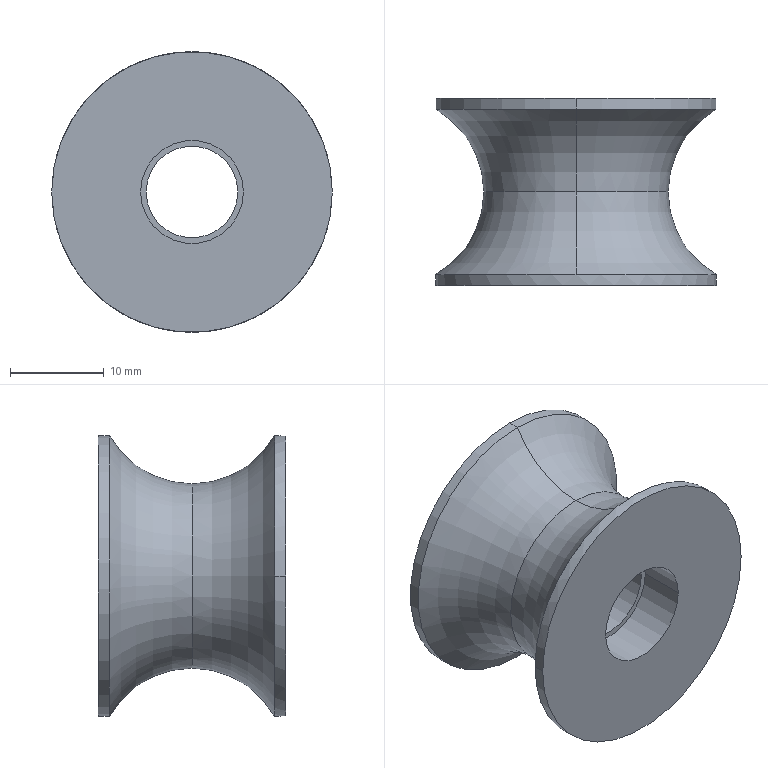Part | STEP file | 06-03 Guide mixing wheel | 1 solid | 18 faces | box 30 x 20 x 30 mm | volume 7202 mm3 | cylinder 10 | torus 4 | plane 4 | commonest cylinder face diameters 11 x4 30 x4 9.8 x2
STEP:
#1=CARTESIAN_POINT('',(0.,0.,0.));
#2=DIRECTION('',(0.,0.,1.));
#3=DIRECTION('',(1.,0.,0.));
#4=AXIS2_PLACEMENT_3D('',#1,#2,#3);
#5=CARTESIAN_POINT('',(0.,8.833,15.));
#6=VERTEX_POINT('',#5);
#7=CARTESIAN_POINT('',(0.,8.833,-15.));
#8=VERTEX_POINT('',#7);
#9=CARTESIAN_POINT('',(0.,8.833,0.));
#10=DIRECTION('',(0.,1.,0.));
#11=DIRECTION('',(-1.,0.,0.));
#12=AXIS2_PLACEMENT_3D('',#9,#10,#11);
#13=CIRCLE('',#12,15.);
#14=CARTESIAN_POINT('',(0.,-0.000000002,0.));
#15=DIRECTION('',(0.,1.,0.));
#16=DIRECTION('',(0.,0.,1.));
#17=AXIS2_PLACEMENT_3D('',#14,#15,#16);
#18=TOROIDAL_SURFACE('',#17,20.,10.15);
#19=CARTESIAN_POINT('',(-1.571,2.086));
#20=DIRECTION('',(1.,0.));
#21=VECTOR('',#20,1.);
#22=LINE('',#19,#21);
#23=(GEOMETRIC_REPRESENTATION_CONTEXT(2)PARAMETRIC_REPRESENTATION_CONTEXT()REPRESENTATION_CONTEXT('',''));
#24=DEFINITIONAL_REPRESENTATION('',(#22),#23);
#25=PCURVE('',#18,#24);
#26=CARTESIAN_POINT('',(0.,8.833,0.));
#27=DIRECTION('',(0.,1.,0.));
#28=DIRECTION('',(0.,0.,1.));
#29=AXIS2_PLACEMENT_3D('',#26,#27,#28);
#30=CYLINDRICAL_SURFACE('',#29,15.);
#31=CARTESIAN_POINT('',(-1.571,-0.000000002));
#32=DIRECTION('',(1.,0.));
#33=VECTOR('',#32,1.);
#34=LINE('',#31,#33);
#35=(GEOMETRIC_REPRESENTATION_CONTEXT(2)PARAMETRIC_REPRESENTATION_CONTEXT()REPRESENTATION_CONTEXT('',''));
#36=DEFINITIONAL_REPRESENTATION('',(#34),#35);
#37=PCURVE('',#30,#36);
#38=SURFACE_CURVE('',#13,(#25,#37),.PCURVE_S1.);
#39=EDGE_CURVE('',#6,#8,#38,.T.);
#40=ORIENTED_EDGE('',*,*,#39,.T.);
#41=CARTESIAN_POINT('',(0.,-0.000000002,-9.85));
#42=VERTEX_POINT('',#41);
#43=CARTESIAN_POINT('',(0.,-0.000000002,-20.));
#44=DIRECTION('',(1.,0.,0.));
#45=DIRECTION('',(0.,0.,-1.));
#46=AXIS2_PLACEMENT_3D('',#43,#44,#45);
#47=CIRCLE('',#46,10.15);
#48=CARTESIAN_POINT('',(3.142,0.));
#49=DIRECTION('',(0.,1.));
#50=VECTOR('',#49,1.);
#51=LINE('',#48,#50);
#52=(GEOMETRIC_REPRESENTATION_CONTEXT(2)PARAMETRIC_REPRESENTATION_CONTEXT()REPRESENTATION_CONTEXT('',''));
#53=DEFINITIONAL_REPRESENTATION('',(#51),#52);
#54=PCURVE('',#18,#53);
#55=CARTESIAN_POINT('',(0.,-0.000000002,0.));
#56=DIRECTION('',(0.,1.,0.));
#57=DIRECTION('',(0.,0.,1.));
#58=AXIS2_PLACEMENT_3D('',#55,#56,#57);
#59=TOROIDAL_SURFACE('',#58,20.,10.15);
#60=CARTESIAN_POINT('',(3.142,0.));
#61=DIRECTION('',(0.,1.));
#62=VECTOR('',#61,1.);
#63=LINE('',#60,#62);
#64=(GEOMETRIC_REPRESENTATION_CONTEXT(2)PARAMETRIC_REPRESENTATION_CONTEXT()REPRESENTATION_CONTEXT('',''));
#65=DEFINITIONAL_REPRESENTATION('',(#63),#64);
#66=PCURVE('',#59,#65);
#67=SURFACE_CURVE('',#47,(#54,#66),.PCURVE_S1.);
#68=EDGE_CURVE('',#8,#42,#67,.T.);
#69=ORIENTED_EDGE('',*,*,#68,.T.);
#70=CARTESIAN_POINT('',(0.,-0.000000002,9.85));
#71=VERTEX_POINT('',#70);
#72=CARTESIAN_POINT('',(0.,-0.000000002,0.));
#73=DIRECTION('',(0.,1.,0.));
#74=DIRECTION('',(0.,0.,1.));
#75=AXIS2_PLACEMENT_3D('',#72,#73,#74);
#76=CIRCLE('',#75,9.85);
#77=CARTESIAN_POINT('',(0.,3.142));
#78=DIRECTION('',(1.,0.));
#79=VECTOR('',#78,1.);
#80=LINE('',#77,#79);
#81=(GEOMETRIC_REPRESENTATION_CONTEXT(2)PARAMETRIC_REPRESENTATION_CONTEXT()REPRESENTATION_CONTEXT('',''));
#82=DEFINITIONAL_REPRESENTATION('',(#80),#81);
#83=PCURVE('',#18,#82);
#84=CARTESIAN_POINT('',(0.,-0.000000002,0.));
#85=DIRECTION('',(0.,1.,0.));
#86=DIRECTION('',(0.,0.,1.));
#87=AXIS2_PLACEMENT_3D('',#84,#85,#86);
#88=TOROIDAL_SURFACE('',#87,20.,10.15);
#89=CARTESIAN_POINT('',(0.,3.142));
#90=DIRECTION('',(1.,0.));
#91=VECTOR('',#90,1.);
#92=LINE('',#89,#91);
#93=(GEOMETRIC_REPRESENTATION_CONTEXT(2)PARAMETRIC_REPRESENTATION_CONTEXT()REPRESENTATION_CONTEXT('',''));
#94=DEFINITIONAL_REPRESENTATION('',(#92),#93);
#95=PCURVE('',#88,#94);
#96=SURFACE_CURVE('',#76,(#83,#95),.PCURVE_S1.);
#97=EDGE_CURVE('',#71,#42,#96,.T.);
#98=ORIENTED_EDGE('',*,*,#97,.F.);
#99=CARTESIAN_POINT('',(0.,-0.000000002,20.));
#100=DIRECTION('',(-1.,0.,0.));
#101=DIRECTION('',(0.,0.,1.));
#102=AXIS2_PLACEMENT_3D('',#99,#100,#101);
#103=CIRCLE('',#102,10.15);
#104=CARTESIAN_POINT('',(0.,0.));
#105=DIRECTION('',(0.,1.));
#106=VECTOR('',#105,1.);
#107=LINE('',#104,#106);
#108=(GEOMETRIC_REPRESENTATION_CONTEXT(2)PARAMETRIC_REPRESENTATION_CONTEXT()REPRESENTATION_CONTEXT('',''));
#109=DEFINITIONAL_REPRESENTATION('',(#107),#108);
#110=PCURVE('',#18,#109);
#111=CARTESIAN_POINT('',(6.283,0.));
#112=DIRECTION('',(0.,1.));
#113=VECTOR('',#112,1.);
#114=LINE('',#111,#113);
#115=(GEOMETRIC_REPRESENTATION_CONTEXT(2)PARAMETRIC_REPRESENTATION_CONTEXT()REPRESENTATION_CONTEXT('',''));
#116=DEFINITIONAL_REPRESENTATION('',(#114),#115);
#117=PCURVE('',#59,#116);
#118=SURFACE_CURVE('',#103,(#110,#117),.PCURVE_S1.);
#119=EDGE_CURVE('',#6,#71,#118,.T.);
#120=ORIENTED_EDGE('',*,*,#119,.F.);
#121=EDGE_LOOP('',(#40,#69,#98,#120));
#122=FACE_BOUND('',#121,.F.);
#123=ADVANCED_FACE('',(#122),#18,.F.);
#124=CARTESIAN_POINT('',(0.,8.833,0.));
#125=DIRECTION('',(0.,1.,0.));
#126=DIRECTION('',(-1.,0.,0.));
#127=AXIS2_PLACEMENT_3D('',#124,#125,#126);
#128=CIRCLE('',#127,15.);
#129=CARTESIAN_POINT('',(-1.571,2.086));
#130=DIRECTION('',(1.,0.));
#131=VECTOR('',#130,1.);
#132=LINE('',#129,#131);
#133=(GEOMETRIC_REPRESENTATION_CONTEXT(2)PARAMETRIC_REPRESENTATION_CONTEXT()REPRESENTATION_CONTEXT('',''));
#134=DEFINITIONAL_REPRESENTATION('',(#132),#133);
#135=PCURVE('',#59,#134);
#136=CARTESIAN_POINT('',(0.,8.833,0.));
#137=DIRECTION('',(0.,1.,0.));
#138=DIRECTION('',(0.,0.,1.));
#139=AXIS2_PLACEMENT_3D('',#136,#137,#138);
#140=CYLINDRICAL_SURFACE('',#139,15.);
#141=CARTESIAN_POINT('',(-1.571,-0.000000002));
#142=DIRECTION('',(1.,0.));
#143=VECTOR('',#142,1.);
#144=LINE('',#141,#143);
#145=(GEOMETRIC_REPRESENTATION_CONTEXT(2)PARAMETRIC_REPRESENTATION_CONTEXT()REPRESENTATION_CONTEXT('',''));
#146=DEFINITIONAL_REPRESENTATION('',(#144),#145);
#147=PCURVE('',#140,#146);
#148=SURFACE_CURVE('',#128,(#135,#147),.PCURVE_S1.);
#149=EDGE_CURVE('',#8,#6,#148,.T.);
#150=ORIENTED_EDGE('',*,*,#149,.T.);
#151=ORIENTED_EDGE('',*,*,#119,.T.);
#152=CARTESIAN_POINT('',(0.,-0.000000002,0.));
#153=DIRECTION('',(0.,1.,0.));
#154=DIRECTION('',(0.,0.,1.));
#155=AXIS2_PLACEMENT_3D('',#152,#153,#154);
#156=CIRCLE('',#155,9.85);
#157=CARTESIAN_POINT('',(0.,3.142));
#158=DIRECTION('',(1.,0.));
#159=VECTOR('',#158,1.);
#160=LINE('',#157,#159);
#161=(GEOMETRIC_REPRESENTATION_CONTEXT(2)PARAMETRIC_REPRESENTATION_CONTEXT()REPRESENTATION_CONTEXT('',''));
#162=DEFINITIONAL_REPRESENTATION('',(#160),#161);
#163=PCURVE('',#59,#162);
#164=CARTESIAN_POINT('',(0.,-0.000000002,0.));
#165=DIRECTION('',(0.,1.,0.));
#166=DIRECTION('',(0.,0.,1.));
#167=AXIS2_PLACEMENT_3D('',#164,#165,#166);
#168=TOROIDAL_SURFACE('',#167,20.,10.15);
#169=CARTESIAN_POINT('',(0.,3.142));
#170=DIRECTION('',(1.,0.));
#171=VECTOR('',#170,1.);
#172=LINE('',#169,#171);
#173=(GEOMETRIC_REPRESENTATION_CONTEXT(2)PARAMETRIC_REPRESENTATION_CONTEXT()REPRESENTATION_CONTEXT('',''));
#174=DEFINITIONAL_REPRESENTATION('',(#172),#173);
#175=PCURVE('',#168,#174);
#176=SURFACE_CURVE('',#156,(#163,#175),.PCURVE_S1.);
#177=EDGE_CURVE('',#42,#71,#176,.T.);
#178=ORIENTED_EDGE('',*,*,#177,.F.);
#179=ORIENTED_EDGE('',*,*,#68,.F.);
#180=EDGE_LOOP('',(#150,#151,#178,#179));
#181=FACE_BOUND('',#180,.F.);
#182=ADVANCED_FACE('',(#181),#59,.F.);
#183=CARTESIAN_POINT('',(0.,-8.833,15.));
#184=VERTEX_POINT('',#183);
#185=CARTESIAN_POINT('',(0.,-0.000000002,20.));
#186=DIRECTION('',(-1.,0.,0.));
#187=DIRECTION('',(0.,0.,1.));
#188=AXIS2_PLACEMENT_3D('',#185,#186,#187);
#189=CIRCLE('',#188,10.15);
#190=CARTESIAN_POINT('',(6.283,0.));
#191=DIRECTION('',(0.,1.));
#192=VECTOR('',#191,1.);
#193=LINE('',#190,#192);
#194=(GEOMETRIC_REPRESENTATION_CONTEXT(2)PARAMETRIC_REPRESENTATION_CONTEXT()REPRESENTATION_CONTEXT('',''));
#195=DEFINITIONAL_REPRESENTATION('',(#193),#194);
#196=PCURVE('',#168,#195);
#197=CARTESIAN_POINT('',(0.,0.));
#198=DIRECTION('',(0.,1.));
#199=VECTOR('',#198,1.);
#200=LINE('',#197,#199);
#201=(GEOMETRIC_REPRESENTATION_CONTEXT(2)PARAMETRIC_REPRESENTATION_CONTEXT()REPRESENTATION_CONTEXT('',''));
#202=DEFINITIONAL_REPRESENTATION('',(#200),#201);
#203=PCURVE('',#88,#202);
#204=SURFACE_CURVE('',#189,(#196,#203),.PCURVE_S1.);
#205=EDGE_CURVE('',#71,#184,#204,.T.);
#206=ORIENTED_EDGE('',*,*,#205,.T.);
#207=CARTESIAN_POINT('',(-15.,-8.833,0.));
#208=VERTEX_POINT('',#207);
#209=CARTESIAN_POINT('',(0.,-8.833,0.));
#210=DIRECTION('',(0.,-1.,0.));
#211=DIRECTION('',(1.,0.,0.));
#212=AXIS2_PLACEMENT_3D('',#209,#210,#211);
#213=CIRCLE('',#212,15.);
#214=CARTESIAN_POINT('',(7.854,4.197));
#215=DIRECTION('',(-1.,0.));
#216=VECTOR('',#215,1.);
#217=LINE('',#214,#216);
#218=(GEOMETRIC_REPRESENTATION_CONTEXT(2)PARAMETRIC_REPRESENTATION_CONTEXT()REPRESENTATION_CONTEXT('',''));
#219=DEFINITIONAL_REPRESENTATION('',(#217),#218);
#220=PCURVE('',#168,#219);
#221=CARTESIAN_POINT('',(0.,-10.,0.));
#222=DIRECTION('',(0.,1.,0.));
#223=DIRECTION('',(-1.,0.,0.));
#224=AXIS2_PLACEMENT_3D('',#221,#222,#223);
#225=CYLINDRICAL_SURFACE('',#224,15.);
#226=CARTESIAN_POINT('',(3.142,1.167));
#227=DIRECTION('',(-1.,0.));
#228=VECTOR('',#227,1.);
#229=LINE('',#226,#228);
#230=(GEOMETRIC_REPRESENTATION_CONTEXT(2)PARAMETRIC_REPRESENTATION_CONTEXT()REPRESENTATION_CONTEXT('',''));
#231=DEFINITIONAL_REPRESENTATION('',(#229),#230);
#232=PCURVE('',#225,#231);
#233=SURFACE_CURVE('',#213,(#220,#232),.PCURVE_S1.);
#234=EDGE_CURVE('',#184,#208,#233,.T.);
#235=ORIENTED_EDGE('',*,*,#234,.T.);
#236=CARTESIAN_POINT('',(0.,-8.833,-15.));
#237=VERTEX_POINT('',#236);
#238=CARTESIAN_POINT('',(0.,-8.833,0.));
#239=DIRECTION('',(0.,-1.,0.));
#240=DIRECTION('',(1.,0.,0.));
#241=AXIS2_PLACEMENT_3D('',#238,#239,#240);
#242=CIRCLE('',#241,15.);
#243=CARTESIAN_POINT('',(7.854,4.197));
#244=DIRECTION('',(-1.,0.));
#245=VECTOR('',#244,1.);
#246=LINE('',#243,#245);
#247=(GEOMETRIC_REPRESENTATION_CONTEXT(2)PARAMETRIC_REPRESENTATION_CONTEXT()REPRESENTATION_CONTEXT('',''));
#248=DEFINITIONAL_REPRESENTATION('',(#246),#247);
#249=PCURVE('',#168,#248);
#250=CARTESIAN_POINT('',(0.,-10.,0.));
#251=DIRECTION('',(0.,1.,0.));
#252=DIRECTION('',(-1.,0.,0.));
#253=AXIS2_PLACEMENT_3D('',#250,#251,#252);
#254=CYLINDRICAL_SURFACE('',#253,15.);
#255=CARTESIAN_POINT('',(9.425,1.167));
#256=DIRECTION('',(-1.,0.));
#257=VECTOR('',#256,1.);
#258=LINE('',#255,#257);
#259=(GEOMETRIC_REPRESENTATION_CONTEXT(2)PARAMETRIC_REPRESENTATION_CONTEXT()REPRESENTATION_CONTEXT('',''));
#260=DEFINITIONAL_REPRESENTATION('',(#258),#259);
#261=PCURVE('',#254,#260);
#262=SURFACE_CURVE('',#242,(#249,#261),.PCURVE_S1.);
#263=EDGE_CURVE('',#208,#237,#262,.T.);
#264=ORIENTED_EDGE('',*,*,#263,.T.);
#265=CARTESIAN_POINT('',(0.,-0.000000002,-20.));
#266=DIRECTION('',(1.,0.,0.));
#267=DIRECTION('',(0.,0.,-1.));
#268=AXIS2_PLACEMENT_3D('',#265,#266,#267);
#269=CIRCLE('',#268,10.15);
#270=CARTESIAN_POINT('',(3.142,0.));
#271=DIRECTION('',(0.,1.));
#272=VECTOR('',#271,1.);
#273=LINE('',#270,#272);
#274=(GEOMETRIC_REPRESENTATION_CONTEXT(2)PARAMETRIC_REPRESENTATION_CONTEXT()REPRESENTATION_CONTEXT('',''));
#275=DEFINITIONAL_REPRESENTATION('',(#273),#274);
#276=PCURVE('',#168,#275);
#277=CARTESIAN_POINT('',(3.142,0.));
#278=DIRECTION('',(0.,1.));
#279=VECTOR('',#278,1.);
#280=LINE('',#277,#279);
#281=(GEOMETRIC_REPRESENTATION_CONTEXT(2)PARAMETRIC_REPRESENTATION_CONTEXT()REPRESENTATION_CONTEXT('',''));
#282=DEFINITIONAL_REPRESENTATION('',(#280),#281);
#283=PCURVE('',#88,#282);
#284=SURFACE_CURVE('',#269,(#276,#283),.PCURVE_S1.);
#285=EDGE_CURVE('',#42,#237,#284,.T.);
#286=ORIENTED_EDGE('',*,*,#285,.F.);
#287=ORIENTED_EDGE('',*,*,#177,.T.);
#288=EDGE_LOOP('',(#206,#235,#264,#286,#287));
#289=FACE_BOUND('',#288,.F.);
#290=ADVANCED_FACE('',(#289),#168,.F.);
#291=ORIENTED_EDGE('',*,*,#39,.T.);
#292=CARTESIAN_POINT('',(0.,10.,-15.));
#293=VERTEX_POINT('',#292);
#294=CARTESIAN_POINT('',(0.,8.833,-15.));
#295=DIRECTION('',(0.,1.,0.));
#296=VECTOR('',#295,1.);
#297=LINE('',#294,#296);
#298=CARTESIAN_POINT('',(3.142,0.));
#299=DIRECTION('',(0.,1.));
#300=VECTOR('',#299,1.);
#301=LINE('',#298,#300);
#302=(GEOMETRIC_REPRESENTATION_CONTEXT(2)PARAMETRIC_REPRESENTATION_CONTEXT()REPRESENTATION_CONTEXT('',''));
#303=DEFINITIONAL_REPRESENTATION('',(#301),#302);
#304=PCURVE('',#30,#303);
#305=CARTESIAN_POINT('',(3.142,0.));
#306=DIRECTION('',(0.,1.));
#307=VECTOR('',#306,1.);
#308=LINE('',#305,#307);
#309=(GEOMETRIC_REPRESENTATION_CONTEXT(2)PARAMETRIC_REPRESENTATION_CONTEXT()REPRESENTATION_CONTEXT('',''));
#310=DEFINITIONAL_REPRESENTATION('',(#308),#309);
#311=PCURVE('',#140,#310);
#312=SURFACE_CURVE('',#297,(#304,#311),.PCURVE_S1.);
#313=EDGE_CURVE('',#8,#293,#312,.T.);
#314=ORIENTED_EDGE('',*,*,#313,.T.);
#315=CARTESIAN_POINT('',(0.,10.,15.));
#316=VERTEX_POINT('',#315);
#317=CARTESIAN_POINT('',(0.,10.,0.));
#318=DIRECTION('',(0.,1.,0.));
#319=DIRECTION('',(0.,0.,1.));
#320=AXIS2_PLACEMENT_3D('',#317,#318,#319);
#321=CIRCLE('',#320,15.);
#322=CARTESIAN_POINT('',(0.,1.167));
#323=DIRECTION('',(1.,0.));
#324=VECTOR('',#323,1.);
#325=LINE('',#322,#324);
#326=(GEOMETRIC_REPRESENTATION_CONTEXT(2)PARAMETRIC_REPRESENTATION_CONTEXT()REPRESENTATION_CONTEXT('',''));
#327=DEFINITIONAL_REPRESENTATION('',(#325),#326);
#328=PCURVE('',#30,#327);
#329=CARTESIAN_POINT('',(-15.18,10.,15.18));
#330=DIRECTION('',(0.,-1.,0.));
#331=DIRECTION('',(0.,0.,-1.));
#332=AXIS2_PLACEMENT_3D('',#329,#330,#331);
#333=PLANE('',#332);
#334=CARTESIAN_POINT('',(0.18,15.18));
#335=CARTESIAN_POINT('',(0.18,41.161));
#336=CARTESIAN_POINT('',(22.68,28.17));
#337=CARTESIAN_POINT('',(45.18,15.18));
#338=CARTESIAN_POINT('',(22.68,2.19));
#339=CARTESIAN_POINT('',(0.18,-10.801));
#340=CARTESIAN_POINT('',(0.18,15.18));
#341=(BOUNDED_CURVE()B_SPLINE_CURVE(2,(#334,#335,#336,#337,#338,#339,#340),.UNSPECIFIED.,.T.,.F.)B_SPLINE_CURVE_WITH_KNOTS((1,2,2,2,2,1),(-2.094,0.,2.094,4.189,6.283,8.378),.UNSPECIFIED.)CURVE()GEOMETRIC_REPRESENTATION_ITEM()RATIONAL_B_SPLINE_CURVE((1.,0.5,1.,0.5,1.,0.5,1.))REPRESENTATION_ITEM(''));
#342=(GEOMETRIC_REPRESENTATION_CONTEXT(2)PARAMETRIC_REPRESENTATION_CONTEXT()REPRESENTATION_CONTEXT('',''));
#343=DEFINITIONAL_REPRESENTATION('',(#341),#342);
#344=PCURVE('',#333,#343);
#345=SURFACE_CURVE('',#321,(#328,#344),.PCURVE_S1.);
#346=EDGE_CURVE('',#316,#293,#345,.T.);
#347=ORIENTED_EDGE('',*,*,#346,.F.);
#348=CARTESIAN_POINT('',(0.,8.833,15.));
#349=DIRECTION('',(0.,1.,0.));
#350=VECTOR('',#349,1.);
#351=LINE('',#348,#350);
#352=CARTESIAN_POINT('',(0.,0.));
#353=DIRECTION('',(0.,1.));
#354=VECTOR('',#353,1.);
#355=LINE('',#352,#354);
#356=(GEOMETRIC_REPRESENTATION_CONTEXT(2)PARAMETRIC_REPRESENTATION_CONTEXT()REPRESENTATION_CONTEXT('',''));
#357=DEFINITIONAL_REPRESENTATION('',(#355),#356);
#358=PCURVE('',#30,#357);
#359=CARTESIAN_POINT('',(6.283,0.));
#360=DIRECTION('',(0.,1.));
#361=VECTOR('',#360,1.);
#362=LINE('',#359,#361);
#363=(GEOMETRIC_REPRESENTATION_CONTEXT(2)PARAMETRIC_REPRESENTATION_CONTEXT()REPRESENTATION_CONTEXT('',''));
#364=DEFINITIONAL_REPRESENTATION('',(#362),#363);
#365=PCURVE('',#140,#364);
#366=SURFACE_CURVE('',#351,(#358,#365),.PCURVE_S1.);
#367=EDGE_CURVE('',#6,#316,#366,.T.);
#368=ORIENTED_EDGE('',*,*,#367,.F.);
#369=EDGE_LOOP('',(#291,#314,#347,#368));
#370=FACE_BOUND('',#369,.T.);
#371=ADVANCED_FACE('',(#370),#30,.T.);
#372=CARTESIAN_POINT('',(15.,-10.,0.));
#373=VERTEX_POINT('',#372);
#374=CARTESIAN_POINT('',(-15.,-10.,0.));
#375=VERTEX_POINT('',#374);
#376=CARTESIAN_POINT('',(0.,-10.,0.));
#377=DIRECTION('',(0.,-1.,0.));
#378=DIRECTION('',(-1.,0.,0.));
#379=AXIS2_PLACEMENT_3D('',#376,#377,#378);
#380=CIRCLE('',#379,15.);
#381=CARTESIAN_POINT('',(6.283,0.));
#382=DIRECTION('',(-1.,0.));
#383=VECTOR('',#382,1.);
#384=LINE('',#381,#383);
#385=(GEOMETRIC_REPRESENTATION_CONTEXT(2)PARAMETRIC_REPRESENTATION_CONTEXT()REPRESENTATION_CONTEXT('',''));
#386=DEFINITIONAL_REPRESENTATION('',(#384),#385);
#387=PCURVE('',#225,#386);
#388=CARTESIAN_POINT('',(-15.18,-10.,-15.18));
#389=DIRECTION('',(0.,1.,0.));
#390=DIRECTION('',(0.,0.,1.));
#391=AXIS2_PLACEMENT_3D('',#388,#389,#390);
#392=PLANE('',#391);
#393=CARTESIAN_POINT('',(15.18,0.18));
#394=CARTESIAN_POINT('',(-10.801,0.18));
#395=CARTESIAN_POINT('',(2.19,22.68));
#396=CARTESIAN_POINT('',(15.18,45.18));
#397=CARTESIAN_POINT('',(28.17,22.68));
#398=CARTESIAN_POINT('',(41.161,0.18));
#399=CARTESIAN_POINT('',(15.18,0.18));
#400=(BOUNDED_CURVE()B_SPLINE_CURVE(2,(#393,#394,#395,#396,#397,#398,#399),.UNSPECIFIED.,.T.,.F.)B_SPLINE_CURVE_WITH_KNOTS((1,2,2,2,2,1),(-2.094,0.,2.094,4.189,6.283,8.378),.UNSPECIFIED.)CURVE()GEOMETRIC_REPRESENTATION_ITEM()RATIONAL_B_SPLINE_CURVE((1.,0.5,1.,0.5,1.,0.5,1.))REPRESENTATION_ITEM(''));
#401=(GEOMETRIC_REPRESENTATION_CONTEXT(2)PARAMETRIC_REPRESENTATION_CONTEXT()REPRESENTATION_CONTEXT('',''));
#402=DEFINITIONAL_REPRESENTATION('',(#400),#401);
#403=PCURVE('',#392,#402);
#404=SURFACE_CURVE('',#380,(#387,#403),.PCURVE_S1.);
#405=EDGE_CURVE('',#373,#375,#404,.T.);
#406=ORIENTED_EDGE('',*,*,#405,.F.);
#407=CARTESIAN_POINT('',(15.,-8.833,0.));
#408=VERTEX_POINT('',#407);
#409=CARTESIAN_POINT('',(15.,-10.,0.));
#410=DIRECTION('',(0.,1.,0.));
#411=VECTOR('',#410,1.);
#412=LINE('',#409,#411);
#413=CARTESIAN_POINT('',(3.142,0.));
#414=DIRECTION('',(0.,1.));
#415=VECTOR('',#414,1.);
#416=LINE('',#413,#415);
#417=(GEOMETRIC_REPRESENTATION_CONTEXT(2)PARAMETRIC_REPRESENTATION_CONTEXT()REPRESENTATION_CONTEXT('',''));
#418=DEFINITIONAL_REPRESENTATION('',(#416),#417);
#419=PCURVE('',#225,#418);
#420=CARTESIAN_POINT('',(3.142,0.));
#421=DIRECTION('',(0.,1.));
#422=VECTOR('',#421,1.);
#423=LINE('',#420,#422);
#424=(GEOMETRIC_REPRESENTATION_CONTEXT(2)PARAMETRIC_REPRESENTATION_CONTEXT()REPRESENTATION_CONTEXT('',''));
#425=DEFINITIONAL_REPRESENTATION('',(#423),#424);
#426=PCURVE('',#254,#425);
#427=SURFACE_CURVE('',#412,(#419,#426),.PCURVE_S1.);
#428=EDGE_CURVE('',#373,#408,#427,.T.);
#429=ORIENTED_EDGE('',*,*,#428,.T.);
#430=CARTESIAN_POINT('',(0.,-8.833,0.));
#431=DIRECTION('',(0.,-1.,0.));
#432=DIRECTION('',(1.,0.,0.));
#433=AXIS2_PLACEMENT_3D('',#430,#431,#432);
#434=CIRCLE('',#433,15.);
#435=CARTESIAN_POINT('',(3.142,1.167));
#436=DIRECTION('',(-1.,0.));
#437=VECTOR('',#436,1.);
#438=LINE('',#435,#437);
#439=(GEOMETRIC_REPRESENTATION_CONTEXT(2)PARAMETRIC_REPRESENTATION_CONTEXT()REPRESENTATION_CONTEXT('',''));
#440=DEFINITIONAL_REPRESENTATION('',(#438),#439);
#441=PCURVE('',#225,#440);
#442=CARTESIAN_POINT('',(1.571,4.197));
#443=DIRECTION('',(-1.,0.));
#444=VECTOR('',#443,1.);
#445=LINE('',#442,#444);
#446=(GEOMETRIC_REPRESENTATION_CONTEXT(2)PARAMETRIC_REPRESENTATION_CONTEXT()REPRESENTATION_CONTEXT('',''));
#447=DEFINITIONAL_REPRESENTATION('',(#445),#446);
#448=PCURVE('',#88,#447);
#449=SURFACE_CURVE('',#434,(#441,#448),.PCURVE_S1.);
#450=EDGE_CURVE('',#408,#184,#449,.T.);
#451=ORIENTED_EDGE('',*,*,#450,.T.);
#452=ORIENTED_EDGE('',*,*,#234,.T.);
#453=CARTESIAN_POINT('',(-15.,-10.,0.));
#454=DIRECTION('',(0.,1.,0.));
#455=VECTOR('',#454,1.);
#456=LINE('',#453,#455);
#457=CARTESIAN_POINT('',(0.,0.));
#458=DIRECTION('',(0.,1.));
#459=VECTOR('',#458,1.);
#460=LINE('',#457,#459);
#461=(GEOMETRIC_REPRESENTATION_CONTEXT(2)PARAMETRIC_REPRESENTATION_CONTEXT()REPRESENTATION_CONTEXT('',''));
#462=DEFINITIONAL_REPRESENTATION('',(#460),#461);
#463=PCURVE('',#225,#462);
#464=CARTESIAN_POINT('',(6.283,0.));
#465=DIRECTION('',(0.,1.));
#466=VECTOR('',#465,1.);
#467=LINE('',#464,#466);
#468=(GEOMETRIC_REPRESENTATION_CONTEXT(2)PARAMETRIC_REPRESENTATION_CONTEXT()REPRESENTATION_CONTEXT('',''));
#469=DEFINITIONAL_REPRESENTATION('',(#467),#468);
#470=PCURVE('',#254,#469);
#471=SURFACE_CURVE('',#456,(#463,#470),.PCURVE_S1.);
#472=EDGE_CURVE('',#375,#208,#471,.T.);
#473=ORIENTED_EDGE('',*,*,#472,.F.);
#474=EDGE_LOOP('',(#406,#429,#451,#452,#473));
#475=FACE_BOUND('',#474,.T.);
#476=ADVANCED_FACE('',(#475),#225,.T.);
#477=CARTESIAN_POINT('',(-5.5,5.,0.));
#478=VERTEX_POINT('',#477);
#479=CARTESIAN_POINT('',(-5.5,10.,0.));
#480=VERTEX_POINT('',#479);
#481=CARTESIAN_POINT('',(-5.5,5.,0.));
#482=DIRECTION('',(0.,1.,0.));
#483=VECTOR('',#482,1.);
#484=LINE('',#481,#483);
#485=CARTESIAN_POINT('',(0.,5.,0.));
#486=DIRECTION('',(0.,1.,0.));
#487=DIRECTION('',(-1.,0.,0.));
#488=AXIS2_PLACEMENT_3D('',#485,#486,#487);
#489=CYLINDRICAL_SURFACE('',#488,5.5);
#490=CARTESIAN_POINT('',(6.283,0.));
#491=DIRECTION('',(0.,1.));
#492=VECTOR('',#491,1.);
#493=LINE('',#490,#492);
#494=(GEOMETRIC_REPRESENTATION_CONTEXT(2)PARAMETRIC_REPRESENTATION_CONTEXT()REPRESENTATION_CONTEXT('',''));
#495=DEFINITIONAL_REPRESENTATION('',(#493),#494);
#496=PCURVE('',#489,#495);
#497=CARTESIAN_POINT('',(0.,5.,0.));
#498=DIRECTION('',(0.,1.,0.));
#499=DIRECTION('',(-1.,0.,0.));
#500=AXIS2_PLACEMENT_3D('',#497,#498,#499);
#501=CYLINDRICAL_SURFACE('',#500,5.5);
#502=CARTESIAN_POINT('',(0.,0.));
#503=DIRECTION('',(0.,1.));
#504=VECTOR('',#503,1.);
#505=LINE('',#502,#504);
#506=(GEOMETRIC_REPRESENTATION_CONTEXT(2)PARAMETRIC_REPRESENTATION_CONTEXT()REPRESENTATION_CONTEXT('',''));
#507=DEFINITIONAL_REPRESENTATION('',(#505),#506);
#508=PCURVE('',#501,#507);
#509=SURFACE_CURVE('',#484,(#496,#508),.PCURVE_S1.);
#510=EDGE_CURVE('',#478,#480,#509,.T.);
#511=ORIENTED_EDGE('',*,*,#510,.T.);
#512=CARTESIAN_POINT('',(5.5,10.,0.));
#513=VERTEX_POINT('',#512);
#514=CARTESIAN_POINT('',(0.,10.,0.));
#515=DIRECTION('',(0.,1.,0.));
#516=DIRECTION('',(-1.,0.,0.));
#517=AXIS2_PLACEMENT_3D('',#514,#515,#516);
#518=CIRCLE('',#517,5.5);
#519=CARTESIAN_POINT('',(0.,5.));
#520=DIRECTION('',(1.,0.));
#521=VECTOR('',#520,1.);
#522=LINE('',#519,#521);
#523=(GEOMETRIC_REPRESENTATION_CONTEXT(2)PARAMETRIC_REPRESENTATION_CONTEXT()REPRESENTATION_CONTEXT('',''));
#524=DEFINITIONAL_REPRESENTATION('',(#522),#523);
#525=PCURVE('',#489,#524);
#526=CARTESIAN_POINT('',(15.18,9.68));
#527=CARTESIAN_POINT('',(5.654,9.68));
#528=CARTESIAN_POINT('',(10.417,17.93));
#529=CARTESIAN_POINT('',(15.18,26.18));
#530=CARTESIAN_POINT('',(19.943,17.93));
#531=CARTESIAN_POINT('',(24.706,9.68));
#532=CARTESIAN_POINT('',(15.18,9.68));
#533=(BOUNDED_CURVE()B_SPLINE_CURVE(2,(#526,#527,#528,#529,#530,#531,#532),.UNSPECIFIED.,.T.,.F.)B_SPLINE_CURVE_WITH_KNOTS((1,2,2,2,2,1),(-2.094,0.,2.094,4.189,6.283,8.378),.UNSPECIFIED.)CURVE()GEOMETRIC_REPRESENTATION_ITEM()RATIONAL_B_SPLINE_CURVE((1.,0.5,1.,0.5,1.,0.5,1.))REPRESENTATION_ITEM(''));
#534=(GEOMETRIC_REPRESENTATION_CONTEXT(2)PARAMETRIC_REPRESENTATION_CONTEXT()REPRESENTATION_CONTEXT('',''));
#535=DEFINITIONAL_REPRESENTATION('',(#533),#534);
#536=PCURVE('',#333,#535);
#537=SURFACE_CURVE('',#518,(#525,#536),.PCURVE_S1.);
#538=EDGE_CURVE('',#513,#480,#537,.T.);
#539=ORIENTED_EDGE('',*,*,#538,.F.);
#540=CARTESIAN_POINT('',(5.5,5.,0.));
#541=VERTEX_POINT('',#540);
#542=CARTESIAN_POINT('',(5.5,5.,0.));
#543=DIRECTION('',(0.,1.,0.));
#544=VECTOR('',#543,1.);
#545=LINE('',#542,#544);
#546=CARTESIAN_POINT('',(3.142,0.));
#547=DIRECTION('',(0.,1.));
#548=VECTOR('',#547,1.);
#549=LINE('',#546,#548);
#550=(GEOMETRIC_REPRESENTATION_CONTEXT(2)PARAMETRIC_REPRESENTATION_CONTEXT()REPRESENTATION_CONTEXT('',''));
#551=DEFINITIONAL_REPRESENTATION('',(#549),#550);
#552=PCURVE('',#489,#551);
#553=CARTESIAN_POINT('',(3.142,0.));
#554=DIRECTION('',(0.,1.));
#555=VECTOR('',#554,1.);
#556=LINE('',#553,#555);
#557=(GEOMETRIC_REPRESENTATION_CONTEXT(2)PARAMETRIC_REPRESENTATION_CONTEXT()REPRESENTATION_CONTEXT('',''));
#558=DEFINITIONAL_REPRESENTATION('',(#556),#557);
#559=PCURVE('',#501,#558);
#560=SURFACE_CURVE('',#545,(#552,#559),.PCURVE_S1.);
#561=EDGE_CURVE('',#541,#513,#560,.T.);
#562=ORIENTED_EDGE('',*,*,#561,.F.);
#563=CARTESIAN_POINT('',(0.,5.,0.));
#564=DIRECTION('',(0.,-1.,0.));
#565=DIRECTION('',(-1.,0.,0.));
#566=AXIS2_PLACEMENT_3D('',#563,#564,#565);
#567=CIRCLE('',#566,5.5);
#568=CARTESIAN_POINT('',(6.283,0.));
#569=DIRECTION('',(-1.,0.));
#570=VECTOR('',#569,1.);
#571=LINE('',#568,#570);
#572=(GEOMETRIC_REPRESENTATION_CONTEXT(2)PARAMETRIC_REPRESENTATION_CONTEXT()REPRESENTATION_CONTEXT('',''));
#573=DEFINITIONAL_REPRESENTATION('',(#571),#572);
#574=PCURVE('',#489,#573);
#575=CARTESIAN_POINT('',(-5.566,5.,5.566));
#576=DIRECTION('',(0.,-1.,0.));
#577=DIRECTION('',(0.,0.,-1.));
#578=AXIS2_PLACEMENT_3D('',#575,#576,#577);
#579=PLANE('',#578);
#580=CARTESIAN_POINT('',(5.566,5.566));
#581=DIRECTION('',(0.,-1.));
#582=AXIS2_PLACEMENT_2D('',#580,#581);
#583=CIRCLE('',#582,5.5);
#584=(GEOMETRIC_REPRESENTATION_CONTEXT(2)PARAMETRIC_REPRESENTATION_CONTEXT()REPRESENTATION_CONTEXT('',''));
#585=DEFINITIONAL_REPRESENTATION('',(#583),#584);
#586=PCURVE('',#579,#585);
#587=SURFACE_CURVE('',#567,(#574,#586),.PCURVE_S1.);
#588=EDGE_CURVE('',#478,#541,#587,.T.);
#589=ORIENTED_EDGE('',*,*,#588,.F.);
#590=EDGE_LOOP('',(#511,#539,#562,#589));
#591=FACE_BOUND('',#590,.F.);
#592=ADVANCED_FACE('',(#591),#489,.F.);
#593=CARTESIAN_POINT('',(-5.5,-10.,0.));
#594=VERTEX_POINT('',#593);
#595=CARTESIAN_POINT('',(-5.5,-5.,0.));
#596=VERTEX_POINT('',#595);
#597=CARTESIAN_POINT('',(-5.5,-10.,0.));
#598=DIRECTION('',(0.,1.,0.));
#599=VECTOR('',#598,1.);
#600=LINE('',#597,#599);
#601=CARTESIAN_POINT('',(0.,-10.,0.));
#602=DIRECTION('',(0.,1.,0.));
#603=DIRECTION('',(-1.,0.,0.));
#604=AXIS2_PLACEMENT_3D('',#601,#602,#603);
#605=CYLINDRICAL_SURFACE('',#604,5.5);
#606=CARTESIAN_POINT('',(6.283,0.));
#607=DIRECTION('',(0.,1.));
#608=VECTOR('',#607,1.);
#609=LINE('',#606,#608);
#610=(GEOMETRIC_REPRESENTATION_CONTEXT(2)PARAMETRIC_REPRESENTATION_CONTEXT()REPRESENTATION_CONTEXT('',''));
#611=DEFINITIONAL_REPRESENTATION('',(#609),#610);
#612=PCURVE('',#605,#611);
#613=CARTESIAN_POINT('',(0.,-10.,0.));
#614=DIRECTION('',(0.,1.,0.));
#615=DIRECTION('',(-1.,0.,0.));
#616=AXIS2_PLACEMENT_3D('',#613,#614,#615);
#617=CYLINDRICAL_SURFACE('',#616,5.5);
#618=CARTESIAN_POINT('',(0.,0.));
#619=DIRECTION('',(0.,1.));
#620=VECTOR('',#619,1.);
#621=LINE('',#618,#620);
#622=(GEOMETRIC_REPRESENTATION_CONTEXT(2)PARAMETRIC_REPRESENTATION_CONTEXT()REPRESENTATION_CONTEXT('',''));
#623=DEFINITIONAL_REPRESENTATION('',(#621),#622);
#624=PCURVE('',#617,#623);
#625=SURFACE_CURVE('',#600,(#612,#624),.PCURVE_S1.);
#626=EDGE_CURVE('',#594,#596,#625,.T.);
#627=ORIENTED_EDGE('',*,*,#626,.T.);
#628=CARTESIAN_POINT('',(5.5,-5.,0.));
#629=VERTEX_POINT('',#628);
#630=CARTESIAN_POINT('',(0.,-5.,0.));
#631=DIRECTION('',(0.,1.,0.));
#632=DIRECTION('',(-1.,0.,0.));
#633=AXIS2_PLACEMENT_3D('',#630,#631,#632);
#634=CIRCLE('',#633,5.5);
#635=CARTESIAN_POINT('',(0.,5.));
#636=DIRECTION('',(1.,0.));
#637=VECTOR('',#636,1.);
#638=LINE('',#635,#637);
#639=(GEOMETRIC_REPRESENTATION_CONTEXT(2)PARAMETRIC_REPRESENTATION_CONTEXT()REPRESENTATION_CONTEXT('',''));
#640=DEFINITIONAL_REPRESENTATION('',(#638),#639);
#641=PCURVE('',#605,#640);
#642=CARTESIAN_POINT('',(-5.566,-5.,-5.566));
#643=DIRECTION('',(0.,1.,0.));
#644=DIRECTION('',(0.,0.,1.));
#645=AXIS2_PLACEMENT_3D('',#642,#643,#644);
#646=PLANE('',#645);
#647=CARTESIAN_POINT('',(5.566,5.566));
#648=DIRECTION('',(0.,-1.));
#649=AXIS2_PLACEMENT_2D('',#647,#648);
#650=CIRCLE('',#649,5.5);
#651=(GEOMETRIC_REPRESENTATION_CONTEXT(2)PARAMETRIC_REPRESENTATION_CONTEXT()REPRESENTATION_CONTEXT('',''));
#652=DEFINITIONAL_REPRESENTATION('',(#650),#651);
#653=PCURVE('',#646,#652);
#654=SURFACE_CURVE('',#634,(#641,#653),.PCURVE_S1.);
#655=EDGE_CURVE('',#629,#596,#654,.T.);
#656=ORIENTED_EDGE('',*,*,#655,.F.);
#657=CARTESIAN_POINT('',(5.5,-10.,0.));
#658=VERTEX_POINT('',#657);
#659=CARTESIAN_POINT('',(5.5,-10.,0.));
#660=DIRECTION('',(0.,1.,0.));
#661=VECTOR('',#660,1.);
#662=LINE('',#659,#661);
#663=CARTESIAN_POINT('',(3.142,0.));
#664=DIRECTION('',(0.,1.));
#665=VECTOR('',#664,1.);
#666=LINE('',#663,#665);
#667=(GEOMETRIC_REPRESENTATION_CONTEXT(2)PARAMETRIC_REPRESENTATION_CONTEXT()REPRESENTATION_CONTEXT('',''));
#668=DEFINITIONAL_REPRESENTATION('',(#666),#667);
#669=PCURVE('',#605,#668);
#670=CARTESIAN_POINT('',(3.142,0.));
#671=DIRECTION('',(0.,1.));
#672=VECTOR('',#671,1.);
#673=LINE('',#670,#672);
#674=(GEOMETRIC_REPRESENTATION_CONTEXT(2)PARAMETRIC_REPRESENTATION_CONTEXT()REPRESENTATION_CONTEXT('',''));
#675=DEFINITIONAL_REPRESENTATION('',(#673),#674);
#676=PCURVE('',#617,#675);
#677=SURFACE_CURVE('',#662,(#669,#676),.PCURVE_S1.);
#678=EDGE_CURVE('',#658,#629,#677,.T.);
#679=ORIENTED_EDGE('',*,*,#678,.F.);
#680=CARTESIAN_POINT('',(0.,-10.,0.));
#681=DIRECTION('',(0.,-1.,0.));
#682=DIRECTION('',(-1.,0.,0.));
#683=AXIS2_PLACEMENT_3D('',#680,#681,#682);
#684=CIRCLE('',#683,5.5);
#685=CARTESIAN_POINT('',(6.283,0.));
#686=DIRECTION('',(-1.,0.));
#687=VECTOR('',#686,1.);
#688=LINE('',#685,#687);
#689=(GEOMETRIC_REPRESENTATION_CONTEXT(2)PARAMETRIC_REPRESENTATION_CONTEXT()REPRESENTATION_CONTEXT('',''));
#690=DEFINITIONAL_REPRESENTATION('',(#688),#689);
#691=PCURVE('',#605,#690);
#692=CARTESIAN_POINT('',(15.18,9.68));
#693=CARTESIAN_POINT('',(5.654,9.68));
#694=CARTESIAN_POINT('',(10.417,17.93));
#695=CARTESIAN_POINT('',(15.18,26.18));
#696=CARTESIAN_POINT('',(19.943,17.93));
#697=CARTESIAN_POINT('',(24.706,9.68));
#698=CARTESIAN_POINT('',(15.18,9.68));
#699=(BOUNDED_CURVE()B_SPLINE_CURVE(2,(#692,#693,#694,#695,#696,#697,#698),.UNSPECIFIED.,.T.,.F.)B_SPLINE_CURVE_WITH_KNOTS((1,2,2,2,2,1),(-2.094,0.,2.094,4.189,6.283,8.378),.UNSPECIFIED.)CURVE()GEOMETRIC_REPRESENTATION_ITEM()RATIONAL_B_SPLINE_CURVE((1.,0.5,1.,0.5,1.,0.5,1.))REPRESENTATION_ITEM(''));
#700=(GEOMETRIC_REPRESENTATION_CONTEXT(2)PARAMETRIC_REPRESENTATION_CONTEXT()REPRESENTATION_CONTEXT('',''));
#701=DEFINITIONAL_REPRESENTATION('',(#699),#700);
#702=PCURVE('',#392,#701);
#703=SURFACE_CURVE('',#684,(#691,#702),.PCURVE_S1.);
#704=EDGE_CURVE('',#594,#658,#703,.T.);
#705=ORIENTED_EDGE('',*,*,#704,.F.);
#706=EDGE_LOOP('',(#627,#656,#679,#705));
#707=FACE_BOUND('',#706,.F.);
#708=ADVANCED_FACE('',(#707),#605,.F.);
#709=CARTESIAN_POINT('',(-4.9,-5.,0.));
#710=VERTEX_POINT('',#709);
#711=CARTESIAN_POINT('',(-4.9,5.,0.));
#712=VERTEX_POINT('',#711);
#713=CARTESIAN_POINT('',(-4.9,-5.,0.));
#714=DIRECTION('',(0.,1.,0.));
#715=VECTOR('',#714,1.);
#716=LINE('',#713,#715);
#717=CARTESIAN_POINT('',(0.,-5.,0.));
#718=DIRECTION('',(0.,1.,0.));
#719=DIRECTION('',(-1.,0.,0.));
#720=AXIS2_PLACEMENT_3D('',#717,#718,#719);
#721=CYLINDRICAL_SURFACE('',#720,4.9);
#722=CARTESIAN_POINT('',(6.283,0.));
#723=DIRECTION('',(0.,1.));
#724=VECTOR('',#723,1.);
#725=LINE('',#722,#724);
#726=(GEOMETRIC_REPRESENTATION_CONTEXT(2)PARAMETRIC_REPRESENTATION_CONTEXT()REPRESENTATION_CONTEXT('',''));
#727=DEFINITIONAL_REPRESENTATION('',(#725),#726);
#728=PCURVE('',#721,#727);
#729=CARTESIAN_POINT('',(0.,-5.,0.));
#730=DIRECTION('',(0.,1.,0.));
#731=DIRECTION('',(-1.,0.,0.));
#732=AXIS2_PLACEMENT_3D('',#729,#730,#731);
#733=CYLINDRICAL_SURFACE('',#732,4.9);
#734=CARTESIAN_POINT('',(0.,0.));
#735=DIRECTION('',(0.,1.));
#736=VECTOR('',#735,1.);
#737=LINE('',#734,#736);
#738=(GEOMETRIC_REPRESENTATION_CONTEXT(2)PARAMETRIC_REPRESENTATION_CONTEXT()REPRESENTATION_CONTEXT('',''));
#739=DEFINITIONAL_REPRESENTATION('',(#737),#738);
#740=PCURVE('',#733,#739);
#741=SURFACE_CURVE('',#716,(#728,#740),.PCURVE_S1.);
#742=EDGE_CURVE('',#710,#712,#741,.T.);
#743=ORIENTED_EDGE('',*,*,#742,.T.);
#744=CARTESIAN_POINT('',(4.9,5.,0.));
#745=VERTEX_POINT('',#744);
#746=CARTESIAN_POINT('',(0.,5.,0.));
#747=DIRECTION('',(0.,1.,0.));
#748=DIRECTION('',(-1.,0.,0.));
#749=AXIS2_PLACEMENT_3D('',#746,#747,#748);
#750=CIRCLE('',#749,4.9);
#751=CARTESIAN_POINT('',(0.,10.));
#752=DIRECTION('',(1.,0.));
#753=VECTOR('',#752,1.);
#754=LINE('',#751,#753);
#755=(GEOMETRIC_REPRESENTATION_CONTEXT(2)PARAMETRIC_REPRESENTATION_CONTEXT()REPRESENTATION_CONTEXT('',''));
#756=DEFINITIONAL_REPRESENTATION('',(#754),#755);
#757=PCURVE('',#721,#756);
#758=CARTESIAN_POINT('',(5.566,0.666));
#759=CARTESIAN_POINT('',(-2.921,0.666));
#760=CARTESIAN_POINT('',(1.322,8.016));
#761=CARTESIAN_POINT('',(5.566,15.366));
#762=CARTESIAN_POINT('',(9.81,8.016));
#763=CARTESIAN_POINT('',(14.053,0.666));
#764=CARTESIAN_POINT('',(5.566,0.666));
#765=(BOUNDED_CURVE()B_SPLINE_CURVE(2,(#758,#759,#760,#761,#762,#763,#764),.UNSPECIFIED.,.T.,.F.)B_SPLINE_CURVE_WITH_KNOTS((1,2,2,2,2,1),(-2.094,0.,2.094,4.189,6.283,8.378),.UNSPECIFIED.)CURVE()GEOMETRIC_REPRESENTATION_ITEM()RATIONAL_B_SPLINE_CURVE((1.,0.5,1.,0.5,1.,0.5,1.))REPRESENTATION_ITEM(''));
#766=(GEOMETRIC_REPRESENTATION_CONTEXT(2)PARAMETRIC_REPRESENTATION_CONTEXT()REPRESENTATION_CONTEXT('',''));
#767=DEFINITIONAL_REPRESENTATION('',(#765),#766);
#768=PCURVE('',#579,#767);
#769=SURFACE_CURVE('',#750,(#757,#768),.PCURVE_S1.);
#770=EDGE_CURVE('',#745,#712,#769,.T.);
#771=ORIENTED_EDGE('',*,*,#770,.F.);
#772=CARTESIAN_POINT('',(4.9,-5.,0.));
#773=VERTEX_POINT('',#772);
#774=CARTESIAN_POINT('',(4.9,-5.,0.));
#775=DIRECTION('',(0.,1.,0.));
#776=VECTOR('',#775,1.);
#777=LINE('',#774,#776);
#778=CARTESIAN_POINT('',(3.142,0.));
#779=DIRECTION('',(0.,1.));
#780=VECTOR('',#779,1.);
#781=LINE('',#778,#780);
#782=(GEOMETRIC_REPRESENTATION_CONTEXT(2)PARAMETRIC_REPRESENTATION_CONTEXT()REPRESENTATION_CONTEXT('',''));
#783=DEFINITIONAL_REPRESENTATION('',(#781),#782);
#784=PCURVE('',#721,#783);
#785=CARTESIAN_POINT('',(3.142,0.));
#786=DIRECTION('',(0.,1.));
#787=VECTOR('',#786,1.);
#788=LINE('',#785,#787);
#789=(GEOMETRIC_REPRESENTATION_CONTEXT(2)PARAMETRIC_REPRESENTATION_CONTEXT()REPRESENTATION_CONTEXT('',''));
#790=DEFINITIONAL_REPRESENTATION('',(#788),#789);
#791=PCURVE('',#733,#790);
#792=SURFACE_CURVE('',#777,(#784,#791),.PCURVE_S1.);
#793=EDGE_CURVE('',#773,#745,#792,.T.);
#794=ORIENTED_EDGE('',*,*,#793,.F.);
#795=CARTESIAN_POINT('',(0.,-5.,0.));
#796=DIRECTION('',(0.,-1.,0.));
#797=DIRECTION('',(-1.,0.,0.));
#798=AXIS2_PLACEMENT_3D('',#795,#796,#797);
#799=CIRCLE('',#798,4.9);
#800=CARTESIAN_POINT('',(6.283,0.));
#801=DIRECTION('',(-1.,0.));
#802=VECTOR('',#801,1.);
#803=LINE('',#800,#802);
#804=(GEOMETRIC_REPRESENTATION_CONTEXT(2)PARAMETRIC_REPRESENTATION_CONTEXT()REPRESENTATION_CONTEXT('',''));
#805=DEFINITIONAL_REPRESENTATION('',(#803),#804);
#806=PCURVE('',#721,#805);
#807=CARTESIAN_POINT('',(5.566,0.666));
#808=CARTESIAN_POINT('',(-2.921,0.666));
#809=CARTESIAN_POINT('',(1.322,8.016));
#810=CARTESIAN_POINT('',(5.566,15.366));
#811=CARTESIAN_POINT('',(9.81,8.016));
#812=CARTESIAN_POINT('',(14.053,0.666));
#813=CARTESIAN_POINT('',(5.566,0.666));
#814=(BOUNDED_CURVE()B_SPLINE_CURVE(2,(#807,#808,#809,#810,#811,#812,#813),.UNSPECIFIED.,.T.,.F.)B_SPLINE_CURVE_WITH_KNOTS((1,2,2,2,2,1),(-2.094,0.,2.094,4.189,6.283,8.378),.UNSPECIFIED.)CURVE()GEOMETRIC_REPRESENTATION_ITEM()RATIONAL_B_SPLINE_CURVE((1.,0.5,1.,0.5,1.,0.5,1.))REPRESENTATION_ITEM(''));
#815=(GEOMETRIC_REPRESENTATION_CONTEXT(2)PARAMETRIC_REPRESENTATION_CONTEXT()REPRESENTATION_CONTEXT('',''));
#816=DEFINITIONAL_REPRESENTATION('',(#814),#815);
#817=PCURVE('',#646,#816);
#818=SURFACE_CURVE('',#799,(#806,#817),.PCURVE_S1.);
#819=EDGE_CURVE('',#710,#773,#818,.T.);
#820=ORIENTED_EDGE('',*,*,#819,.F.);
#821=EDGE_LOOP('',(#743,#771,#794,#820));
#822=FACE_BOUND('',#821,.F.);
#823=ADVANCED_FACE('',(#822),#721,.F.);
#824=ORIENTED_EDGE('',*,*,#285,.T.);
#825=CARTESIAN_POINT('',(0.,-8.833,0.));
#826=DIRECTION('',(0.,-1.,0.));
#827=DIRECTION('',(1.,0.,0.));
#828=AXIS2_PLACEMENT_3D('',#825,#826,#827);
#829=CIRCLE('',#828,15.);
#830=CARTESIAN_POINT('',(7.854,4.197));
#831=DIRECTION('',(-1.,0.));
#832=VECTOR('',#831,1.);
#833=LINE('',#830,#832);
#834=(GEOMETRIC_REPRESENTATION_CONTEXT(2)PARAMETRIC_REPRESENTATION_CONTEXT()REPRESENTATION_CONTEXT('',''));
#835=DEFINITIONAL_REPRESENTATION('',(#833),#834);
#836=PCURVE('',#88,#835);
#837=CARTESIAN_POINT('',(9.425,1.167));
#838=DIRECTION('',(-1.,0.));
#839=VECTOR('',#838,1.);
#840=LINE('',#837,#839);
#841=(GEOMETRIC_REPRESENTATION_CONTEXT(2)PARAMETRIC_REPRESENTATION_CONTEXT()REPRESENTATION_CONTEXT('',''));
#842=DEFINITIONAL_REPRESENTATION('',(#840),#841);
#843=PCURVE('',#254,#842);
#844=SURFACE_CURVE('',#829,(#836,#843),.PCURVE_S1.);
#845=EDGE_CURVE('',#237,#408,#844,.T.);
#846=ORIENTED_EDGE('',*,*,#845,.T.);
#847=ORIENTED_EDGE('',*,*,#450,.T.);
#848=ORIENTED_EDGE('',*,*,#205,.F.);
#849=ORIENTED_EDGE('',*,*,#97,.T.);
#850=EDGE_LOOP('',(#824,#846,#847,#848,#849));
#851=FACE_BOUND('',#850,.F.);
#852=ADVANCED_FACE('',(#851),#88,.F.);
#853=ORIENTED_EDGE('',*,*,#313,.F.);
#854=ORIENTED_EDGE('',*,*,#149,.T.);
#855=ORIENTED_EDGE('',*,*,#367,.T.);
#856=CARTESIAN_POINT('',(0.,10.,0.));
#857=DIRECTION('',(0.,1.,0.));
#858=DIRECTION('',(0.,0.,1.));
#859=AXIS2_PLACEMENT_3D('',#856,#857,#858);
#860=CIRCLE('',#859,15.);
#861=CARTESIAN_POINT('',(0.,1.167));
#862=DIRECTION('',(1.,0.));
#863=VECTOR('',#862,1.);
#864=LINE('',#861,#863);
#865=(GEOMETRIC_REPRESENTATION_CONTEXT(2)PARAMETRIC_REPRESENTATION_CONTEXT()REPRESENTATION_CONTEXT('',''));
#866=DEFINITIONAL_REPRESENTATION('',(#864),#865);
#867=PCURVE('',#140,#866);
#868=CARTESIAN_POINT('',(0.18,15.18));
#869=CARTESIAN_POINT('',(0.18,41.161));
#870=CARTESIAN_POINT('',(22.68,28.17));
#871=CARTESIAN_POINT('',(45.18,15.18));
#872=CARTESIAN_POINT('',(22.68,2.19));
#873=CARTESIAN_POINT('',(0.18,-10.801));
#874=CARTESIAN_POINT('',(0.18,15.18));
#875=(BOUNDED_CURVE()B_SPLINE_CURVE(2,(#868,#869,#870,#871,#872,#873,#874),.UNSPECIFIED.,.T.,.F.)B_SPLINE_CURVE_WITH_KNOTS((1,2,2,2,2,1),(-2.094,0.,2.094,4.189,6.283,8.378),.UNSPECIFIED.)CURVE()GEOMETRIC_REPRESENTATION_ITEM()RATIONAL_B_SPLINE_CURVE((1.,0.5,1.,0.5,1.,0.5,1.))REPRESENTATION_ITEM(''));
#876=(GEOMETRIC_REPRESENTATION_CONTEXT(2)PARAMETRIC_REPRESENTATION_CONTEXT()REPRESENTATION_CONTEXT('',''));
#877=DEFINITIONAL_REPRESENTATION('',(#875),#876);
#878=PCURVE('',#333,#877);
#879=SURFACE_CURVE('',#860,(#867,#878),.PCURVE_S1.);
#880=EDGE_CURVE('',#293,#316,#879,.T.);
#881=ORIENTED_EDGE('',*,*,#880,.F.);
#882=EDGE_LOOP('',(#853,#854,#855,#881));
#883=FACE_BOUND('',#882,.T.);
#884=ADVANCED_FACE('',(#883),#140,.T.);
#885=ORIENTED_EDGE('',*,*,#428,.F.);
#886=CARTESIAN_POINT('',(0.,-10.,0.));
#887=DIRECTION('',(0.,-1.,0.));
#888=DIRECTION('',(-1.,0.,0.));
#889=AXIS2_PLACEMENT_3D('',#886,#887,#888);
#890=CIRCLE('',#889,15.);
#891=CARTESIAN_POINT('',(6.283,0.));
#892=DIRECTION('',(-1.,0.));
#893=VECTOR('',#892,1.);
#894=LINE('',#891,#893);
#895=(GEOMETRIC_REPRESENTATION_CONTEXT(2)PARAMETRIC_REPRESENTATION_CONTEXT()REPRESENTATION_CONTEXT('',''));
#896=DEFINITIONAL_REPRESENTATION('',(#894),#895);
#897=PCURVE('',#254,#896);
#898=CARTESIAN_POINT('',(15.18,0.18));
#899=CARTESIAN_POINT('',(-10.801,0.18));
#900=CARTESIAN_POINT('',(2.19,22.68));
#901=CARTESIAN_POINT('',(15.18,45.18));
#902=CARTESIAN_POINT('',(28.17,22.68));
#903=CARTESIAN_POINT('',(41.161,0.18));
#904=CARTESIAN_POINT('',(15.18,0.18));
#905=(BOUNDED_CURVE()B_SPLINE_CURVE(2,(#898,#899,#900,#901,#902,#903,#904),.UNSPECIFIED.,.T.,.F.)B_SPLINE_CURVE_WITH_KNOTS((1,2,2,2,2,1),(-2.094,0.,2.094,4.189,6.283,8.378),.UNSPECIFIED.)CURVE()GEOMETRIC_REPRESENTATION_ITEM()RATIONAL_B_SPLINE_CURVE((1.,0.5,1.,0.5,1.,0.5,1.))REPRESENTATION_ITEM(''));
#906=(GEOMETRIC_REPRESENTATION_CONTEXT(2)PARAMETRIC_REPRESENTATION_CONTEXT()REPRESENTATION_CONTEXT('',''));
#907=DEFINITIONAL_REPRESENTATION('',(#905),#906);
#908=PCURVE('',#392,#907);
#909=SURFACE_CURVE('',#890,(#897,#908),.PCURVE_S1.);
#910=EDGE_CURVE('',#375,#373,#909,.T.);
#911=ORIENTED_EDGE('',*,*,#910,.F.);
#912=ORIENTED_EDGE('',*,*,#472,.T.);
#913=ORIENTED_EDGE('',*,*,#263,.T.);
#914=ORIENTED_EDGE('',*,*,#845,.T.);
#915=EDGE_LOOP('',(#885,#911,#912,#913,#914));
#916=FACE_BOUND('',#915,.T.);
#917=ADVANCED_FACE('',(#916),#254,.T.);
#918=CARTESIAN_POINT('',(0.,10.,0.));
#919=DIRECTION('',(0.,1.,0.));
#920=DIRECTION('',(-1.,0.,0.));
#921=AXIS2_PLACEMENT_3D('',#918,#919,#920);
#922=CIRCLE('',#921,5.5);
#923=CARTESIAN_POINT('',(15.18,9.68));
#924=CARTESIAN_POINT('',(5.654,9.68));
#925=CARTESIAN_POINT('',(10.417,17.93));
#926=CARTESIAN_POINT('',(15.18,26.18));
#927=CARTESIAN_POINT('',(19.943,17.93));
#928=CARTESIAN_POINT('',(24.706,9.68));
#929=CARTESIAN_POINT('',(15.18,9.68));
#930=(BOUNDED_CURVE()B_SPLINE_CURVE(2,(#923,#924,#925,#926,#927,#928,#929),.UNSPECIFIED.,.T.,.F.)B_SPLINE_CURVE_WITH_KNOTS((1,2,2,2,2,1),(-2.094,0.,2.094,4.189,6.283,8.378),.UNSPECIFIED.)CURVE()GEOMETRIC_REPRESENTATION_ITEM()RATIONAL_B_SPLINE_CURVE((1.,0.5,1.,0.5,1.,0.5,1.))REPRESENTATION_ITEM(''));
#931=(GEOMETRIC_REPRESENTATION_CONTEXT(2)PARAMETRIC_REPRESENTATION_CONTEXT()REPRESENTATION_CONTEXT('',''));
#932=DEFINITIONAL_REPRESENTATION('',(#930),#931);
#933=PCURVE('',#333,#932);
#934=CARTESIAN_POINT('',(0.,5.));
#935=DIRECTION('',(1.,0.));
#936=VECTOR('',#935,1.);
#937=LINE('',#934,#936);
#938=(GEOMETRIC_REPRESENTATION_CONTEXT(2)PARAMETRIC_REPRESENTATION_CONTEXT()REPRESENTATION_CONTEXT('',''));
#939=DEFINITIONAL_REPRESENTATION('',(#937),#938);
#940=PCURVE('',#501,#939);
#941=SURFACE_CURVE('',#922,(#933,#940),.PCURVE_S1.);
#942=EDGE_CURVE('',#480,#513,#941,.T.);
#943=ORIENTED_EDGE('',*,*,#942,.F.);
#944=ORIENTED_EDGE('',*,*,#538,.F.);
#945=EDGE_LOOP('',(#943,#944));
#946=FACE_BOUND('',#945,.T.);
#947=ORIENTED_EDGE('',*,*,#346,.T.);
#948=ORIENTED_EDGE('',*,*,#880,.T.);
#949=EDGE_LOOP('',(#947,#948));
#950=FACE_BOUND('',#949,.T.);
#951=ADVANCED_FACE('',(#946,#950),#333,.F.);
#952=ORIENTED_EDGE('',*,*,#704,.F.);
#953=CARTESIAN_POINT('',(0.,-10.,0.));
#954=DIRECTION('',(0.,-1.,0.));
#955=DIRECTION('',(-1.,0.,0.));
#956=AXIS2_PLACEMENT_3D('',#953,#954,#955);
#957=CIRCLE('',#956,5.5);
#958=CARTESIAN_POINT('',(15.18,9.68));
#959=CARTESIAN_POINT('',(5.654,9.68));
#960=CARTESIAN_POINT('',(10.417,17.93));
#961=CARTESIAN_POINT('',(15.18,26.18));
#962=CARTESIAN_POINT('',(19.943,17.93));
#963=CARTESIAN_POINT('',(24.706,9.68));
#964=CARTESIAN_POINT('',(15.18,9.68));
#965=(BOUNDED_CURVE()B_SPLINE_CURVE(2,(#958,#959,#960,#961,#962,#963,#964),.UNSPECIFIED.,.T.,.F.)B_SPLINE_CURVE_WITH_KNOTS((1,2,2,2,2,1),(-2.094,0.,2.094,4.189,6.283,8.378),.UNSPECIFIED.)CURVE()GEOMETRIC_REPRESENTATION_ITEM()RATIONAL_B_SPLINE_CURVE((1.,0.5,1.,0.5,1.,0.5,1.))REPRESENTATION_ITEM(''));
#966=(GEOMETRIC_REPRESENTATION_CONTEXT(2)PARAMETRIC_REPRESENTATION_CONTEXT()REPRESENTATION_CONTEXT('',''));
#967=DEFINITIONAL_REPRESENTATION('',(#965),#966);
#968=PCURVE('',#392,#967);
#969=CARTESIAN_POINT('',(6.283,0.));
#970=DIRECTION('',(-1.,0.));
#971=VECTOR('',#970,1.);
#972=LINE('',#969,#971);
#973=(GEOMETRIC_REPRESENTATION_CONTEXT(2)PARAMETRIC_REPRESENTATION_CONTEXT()REPRESENTATION_CONTEXT('',''));
#974=DEFINITIONAL_REPRESENTATION('',(#972),#973);
#975=PCURVE('',#617,#974);
#976=SURFACE_CURVE('',#957,(#968,#975),.PCURVE_S1.);
#977=EDGE_CURVE('',#658,#594,#976,.T.);
#978=ORIENTED_EDGE('',*,*,#977,.F.);
#979=EDGE_LOOP('',(#952,#978));
#980=FACE_BOUND('',#979,.T.);
#981=ORIENTED_EDGE('',*,*,#910,.T.);
#982=ORIENTED_EDGE('',*,*,#405,.T.);
#983=EDGE_LOOP('',(#981,#982));
#984=FACE_BOUND('',#983,.T.);
#985=ADVANCED_FACE('',(#980,#984),#392,.F.);
#986=ORIENTED_EDGE('',*,*,#942,.F.);
#987=ORIENTED_EDGE('',*,*,#510,.F.);
#988=CARTESIAN_POINT('',(0.,5.,0.));
#989=DIRECTION('',(0.,-1.,0.));
#990=DIRECTION('',(-1.,0.,0.));
#991=AXIS2_PLACEMENT_3D('',#988,#989,#990);
#992=CIRCLE('',#991,5.5);
#993=CARTESIAN_POINT('',(6.283,0.));
#994=DIRECTION('',(-1.,0.));
#995=VECTOR('',#994,1.);
#996=LINE('',#993,#995);
#997=(GEOMETRIC_REPRESENTATION_CONTEXT(2)PARAMETRIC_REPRESENTATION_CONTEXT()REPRESENTATION_CONTEXT('',''));
#998=DEFINITIONAL_REPRESENTATION('',(#996),#997);
#999=PCURVE('',#501,#998);
#1000=CARTESIAN_POINT('',(5.566,5.566));
#1001=DIRECTION('',(0.,-1.));
#1002=AXIS2_PLACEMENT_2D('',#1000,#1001);
#1003=CIRCLE('',#1002,5.5);
#1004=(GEOMETRIC_REPRESENTATION_CONTEXT(2)PARAMETRIC_REPRESENTATION_CONTEXT()REPRESENTATION_CONTEXT('',''));
#1005=DEFINITIONAL_REPRESENTATION('',(#1003),#1004);
#1006=PCURVE('',#579,#1005);
#1007=SURFACE_CURVE('',#992,(#999,#1006),.PCURVE_S1.);
#1008=EDGE_CURVE('',#541,#478,#1007,.T.);
#1009=ORIENTED_EDGE('',*,*,#1008,.F.);
#1010=ORIENTED_EDGE('',*,*,#561,.T.);
#1011=EDGE_LOOP('',(#986,#987,#1009,#1010));
#1012=FACE_BOUND('',#1011,.F.);
#1013=ADVANCED_FACE('',(#1012),#501,.F.);
#1014=CARTESIAN_POINT('',(0.,-5.,0.));
#1015=DIRECTION('',(0.,1.,0.));
#1016=DIRECTION('',(-1.,0.,0.));
#1017=AXIS2_PLACEMENT_3D('',#1014,#1015,#1016);
#1018=CIRCLE('',#1017,5.5);
#1019=CARTESIAN_POINT('',(0.,5.));
#1020=DIRECTION('',(1.,0.));
#1021=VECTOR('',#1020,1.);
#1022=LINE('',#1019,#1021);
#1023=(GEOMETRIC_REPRESENTATION_CONTEXT(2)PARAMETRIC_REPRESENTATION_CONTEXT()REPRESENTATION_CONTEXT('',''));
#1024=DEFINITIONAL_REPRESENTATION('',(#1022),#1023);
#1025=PCURVE('',#617,#1024);
#1026=CARTESIAN_POINT('',(5.566,5.566));
#1027=DIRECTION('',(0.,-1.));
#1028=AXIS2_PLACEMENT_2D('',#1026,#1027);
#1029=CIRCLE('',#1028,5.5);
#1030=(GEOMETRIC_REPRESENTATION_CONTEXT(2)PARAMETRIC_REPRESENTATION_CONTEXT()REPRESENTATION_CONTEXT('',''));
#1031=DEFINITIONAL_REPRESENTATION('',(#1029),#1030);
#1032=PCURVE('',#646,#1031);
#1033=SURFACE_CURVE('',#1018,(#1025,#1032),.PCURVE_S1.);
#1034=EDGE_CURVE('',#596,#629,#1033,.T.);
#1035=ORIENTED_EDGE('',*,*,#1034,.F.);
#1036=ORIENTED_EDGE('',*,*,#626,.F.);
#1037=ORIENTED_EDGE('',*,*,#977,.F.);
#1038=ORIENTED_EDGE('',*,*,#678,.T.);
#1039=EDGE_LOOP('',(#1035,#1036,#1037,#1038));
#1040=FACE_BOUND('',#1039,.F.);
#1041=ADVANCED_FACE('',(#1040),#617,.F.);
#1042=CARTESIAN_POINT('',(0.,5.,0.));
#1043=DIRECTION('',(0.,1.,0.));
#1044=DIRECTION('',(-1.,0.,0.));
#1045=AXIS2_PLACEMENT_3D('',#1042,#1043,#1044);
#1046=CIRCLE('',#1045,4.9);
#1047=CARTESIAN_POINT('',(5.566,0.666));
#1048=CARTESIAN_POINT('',(-2.921,0.666));
#1049=CARTESIAN_POINT('',(1.322,8.016));
#1050=CARTESIAN_POINT('',(5.566,15.366));
#1051=CARTESIAN_POINT('',(9.81,8.016));
#1052=CARTESIAN_POINT('',(14.053,0.666));
#1053=CARTESIAN_POINT('',(5.566,0.666));
#1054=(BOUNDED_CURVE()B_SPLINE_CURVE(2,(#1047,#1048,#1049,#1050,#1051,#1052,#1053),.UNSPECIFIED.,.T.,.F.)B_SPLINE_CURVE_WITH_KNOTS((1,2,2,2,2,1),(-2.094,0.,2.094,4.189,6.283,8.378),.UNSPECIFIED.)CURVE()GEOMETRIC_REPRESENTATION_ITEM()RATIONAL_B_SPLINE_CURVE((1.,0.5,1.,0.5,1.,0.5,1.))REPRESENTATION_ITEM(''));
#1055=(GEOMETRIC_REPRESENTATION_CONTEXT(2)PARAMETRIC_REPRESENTATION_CONTEXT()REPRESENTATION_CONTEXT('',''));
#1056=DEFINITIONAL_REPRESENTATION('',(#1054),#1055);
#1057=PCURVE('',#579,#1056);
#1058=CARTESIAN_POINT('',(0.,10.));
#1059=DIRECTION('',(1.,0.));
#1060=VECTOR('',#1059,1.);
#1061=LINE('',#1058,#1060);
#1062=(GEOMETRIC_REPRESENTATION_CONTEXT(2)PARAMETRIC_REPRESENTATION_CONTEXT()REPRESENTATION_CONTEXT('',''));
#1063=DEFINITIONAL_REPRESENTATION('',(#1061),#1062);
#1064=PCURVE('',#733,#1063);
#1065=SURFACE_CURVE('',#1046,(#1057,#1064),.PCURVE_S1.);
#1066=EDGE_CURVE('',#712,#745,#1065,.T.);
#1067=ORIENTED_EDGE('',*,*,#1066,.F.);
#1068=ORIENTED_EDGE('',*,*,#770,.F.);
#1069=EDGE_LOOP('',(#1067,#1068));
#1070=FACE_BOUND('',#1069,.T.);
#1071=ORIENTED_EDGE('',*,*,#588,.F.);
#1072=ORIENTED_EDGE('',*,*,#1008,.F.);
#1073=EDGE_LOOP('',(#1071,#1072));
#1074=FACE_BOUND('',#1073,.T.);
#1075=ADVANCED_FACE('',(#1070,#1074),#579,.F.);
#1076=ORIENTED_EDGE('',*,*,#819,.F.);
#1077=CARTESIAN_POINT('',(0.,-5.,0.));
#1078=DIRECTION('',(0.,-1.,0.));
#1079=DIRECTION('',(-1.,0.,0.));
#1080=AXIS2_PLACEMENT_3D('',#1077,#1078,#1079);
#1081=CIRCLE('',#1080,4.9);
#1082=CARTESIAN_POINT('',(5.566,0.666));
#1083=CARTESIAN_POINT('',(-2.921,0.666));
#1084=CARTESIAN_POINT('',(1.322,8.016));
#1085=CARTESIAN_POINT('',(5.566,15.366));
#1086=CARTESIAN_POINT('',(9.81,8.016));
#1087=CARTESIAN_POINT('',(14.053,0.666));
#1088=CARTESIAN_POINT('',(5.566,0.666));
#1089=(BOUNDED_CURVE()B_SPLINE_CURVE(2,(#1082,#1083,#1084,#1085,#1086,#1087,#1088),.UNSPECIFIED.,.T.,.F.)B_SPLINE_CURVE_WITH_KNOTS((1,2,2,2,2,1),(-2.094,0.,2.094,4.189,6.283,8.378),.UNSPECIFIED.)CURVE()GEOMETRIC_REPRESENTATION_ITEM()RATIONAL_B_SPLINE_CURVE((1.,0.5,1.,0.5,1.,0.5,1.))REPRESENTATION_ITEM(''));
#1090=(GEOMETRIC_REPRESENTATION_CONTEXT(2)PARAMETRIC_REPRESENTATION_CONTEXT()REPRESENTATION_CONTEXT('',''));
#1091=DEFINITIONAL_REPRESENTATION('',(#1089),#1090);
#1092=PCURVE('',#646,#1091);
#1093=CARTESIAN_POINT('',(6.283,0.));
#1094=DIRECTION('',(-1.,0.));
#1095=VECTOR('',#1094,1.);
#1096=LINE('',#1093,#1095);
#1097=(GEOMETRIC_REPRESENTATION_CONTEXT(2)PARAMETRIC_REPRESENTATION_CONTEXT()REPRESENTATION_CONTEXT('',''));
#1098=DEFINITIONAL_REPRESENTATION('',(#1096),#1097);
#1099=PCURVE('',#733,#1098);
#1100=SURFACE_CURVE('',#1081,(#1092,#1099),.PCURVE_S1.);
#1101=EDGE_CURVE('',#773,#710,#1100,.T.);
#1102=ORIENTED_EDGE('',*,*,#1101,.F.);
#1103=EDGE_LOOP('',(#1076,#1102));
#1104=FACE_BOUND('',#1103,.T.);
#1105=ORIENTED_EDGE('',*,*,#1034,.F.);
#1106=ORIENTED_EDGE('',*,*,#655,.F.);
#1107=EDGE_LOOP('',(#1105,#1106));
#1108=FACE_BOUND('',#1107,.T.);
#1109=ADVANCED_FACE('',(#1104,#1108),#646,.F.);
#1110=ORIENTED_EDGE('',*,*,#1066,.F.);
#1111=ORIENTED_EDGE('',*,*,#742,.F.);
#1112=ORIENTED_EDGE('',*,*,#1101,.F.);
#1113=ORIENTED_EDGE('',*,*,#793,.T.);
#1114=EDGE_LOOP('',(#1110,#1111,#1112,#1113));
#1115=FACE_BOUND('',#1114,.F.);
#1116=ADVANCED_FACE('',(#1115),#733,.F.);
#1117=CLOSED_SHELL('',(#123,#182,#290,#371,#476,#592,#708,#823,#852,#884,#917,#951,#985,#1013,#1041,#1075,#1109,#1116));
#1118=MANIFOLD_SOLID_BREP('',#1117);
#1119=(LENGTH_UNIT()NAMED_UNIT(*)SI_UNIT(.MILLI.,.METRE.));
#1120=UNCERTAINTY_MEASURE_WITH_UNIT(LENGTH_MEASURE(0.0000001),#1119,'','');
#1121=(NAMED_UNIT(*)PLANE_ANGLE_UNIT()SI_UNIT($,.RADIAN.));
#1122=(NAMED_UNIT(*)SI_UNIT($,.STERADIAN.)SOLID_ANGLE_UNIT());
#1123=(GEOMETRIC_REPRESENTATION_CONTEXT(3)GLOBAL_UNCERTAINTY_ASSIGNED_CONTEXT((#1120))GLOBAL_UNIT_ASSIGNED_CONTEXT((#1119,#1121,#1122))REPRESENTATION_CONTEXT('',''));
#1124=ADVANCED_BREP_SHAPE_REPRESENTATION('',(#4,#1118),#1123);